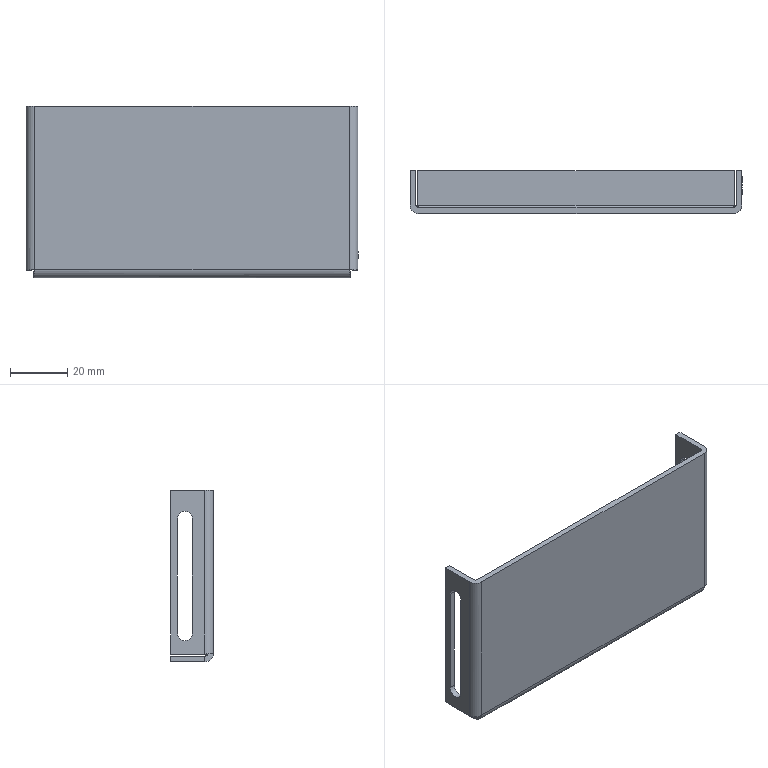Part | SolidWorks | features BaseBody 1 | 1 solid | 34 faces | box 116 x 15 x 60 mm | volume 18438 mm3 | plane 20 | cylinder 10 | spline 4 | commonest cylinder face diameters 5.2 x4 2 x3 6 x3
STEP:
#1=CARTESIAN_POINT('',(-114.,5.4,-10.));
#2=VERTEX_POINT('',#1);
#3=CARTESIAN_POINT('',(-114.,10.6,-10.));
#4=VERTEX_POINT('',#3);
#5=CARTESIAN_POINT('',(-114.,8.,-10.));
#6=DIRECTION('',(-1.,0.,0.));
#7=DIRECTION('',(0.,-1.,0.));
#8=AXIS2_PLACEMENT_3D('',#5,#6,#7);
#9=CIRCLE('',#8,2.6);
#10=EDGE_CURVE('',#2,#4,#9,.T.);
#11=ORIENTED_EDGE('',*,*,#10,.T.);
#12=CARTESIAN_POINT('',(-114.,10.6,-50.));
#13=VERTEX_POINT('',#12);
#14=CARTESIAN_POINT('',(-114.,10.6,-50.));
#15=DIRECTION('',(0.,0.,-1.));
#16=VECTOR('',#15,1000.);
#17=LINE('',#14,#16);
#18=EDGE_CURVE('',#4,#13,#17,.T.);
#19=ORIENTED_EDGE('',*,*,#18,.T.);
#20=CARTESIAN_POINT('',(-114.,5.4,-50.));
#21=VERTEX_POINT('',#20);
#22=CARTESIAN_POINT('',(-114.,8.,-50.));
#23=DIRECTION('',(-1.,0.,0.));
#24=DIRECTION('',(0.,-1.,0.));
#25=AXIS2_PLACEMENT_3D('',#22,#23,#24);
#26=CIRCLE('',#25,2.6);
#27=EDGE_CURVE('',#13,#21,#26,.T.);
#28=ORIENTED_EDGE('',*,*,#27,.T.);
#29=CARTESIAN_POINT('',(-114.,5.4,-50.));
#30=DIRECTION('',(0.,0.,1.));
#31=VECTOR('',#30,1000.);
#32=LINE('',#29,#31);
#33=EDGE_CURVE('',#21,#2,#32,.T.);
#34=ORIENTED_EDGE('',*,*,#33,.T.);
#35=EDGE_LOOP('',(#11,#19,#28,#34));
#36=FACE_BOUND('',#35,.T.);
#37=CARTESIAN_POINT('',(-114.,13.,-57.293));
#38=VERTEX_POINT('',#37);
#39=CARTESIAN_POINT('',(-114.,13.,0.));
#40=VERTEX_POINT('',#39);
#41=CARTESIAN_POINT('',(-114.,13.,-60.));
#42=DIRECTION('',(0.,0.,1.));
#43=VECTOR('',#42,1000.);
#44=LINE('',#41,#43);
#45=EDGE_CURVE('',#38,#40,#44,.T.);
#46=ORIENTED_EDGE('',*,*,#45,.T.);
#47=CARTESIAN_POINT('',(-114.,1.,0.));
#48=VERTEX_POINT('',#47);
#49=CARTESIAN_POINT('',(-114.,13.,0.));
#50=DIRECTION('',(0.,-1.,0.));
#51=VECTOR('',#50,1000.);
#52=LINE('',#49,#51);
#53=EDGE_CURVE('',#40,#48,#52,.T.);
#54=ORIENTED_EDGE('',*,*,#53,.T.);
#55=CARTESIAN_POINT('',(-114.,1.,-57.293));
#56=VERTEX_POINT('',#55);
#57=CARTESIAN_POINT('',(-114.,1.,0.));
#58=DIRECTION('',(0.,0.,-1.));
#59=VECTOR('',#58,1000.);
#60=LINE('',#57,#59);
#61=EDGE_CURVE('',#48,#56,#60,.T.);
#62=ORIENTED_EDGE('',*,*,#61,.T.);
#63=CARTESIAN_POINT('',(-114.,0.,-57.293));
#64=DIRECTION('',(0.,-1.,0.));
#65=VECTOR('',#64,1000.);
#66=LINE('',#63,#65);
#67=EDGE_CURVE('',#38,#56,#66,.T.);
#68=ORIENTED_EDGE('',*,*,#67,.F.);
#69=EDGE_LOOP('',(#46,#54,#62,#68));
#70=FACE_OUTER_BOUND('',#69,.T.);
#71=CARTESIAN_POINT('',(-114.,0.,0.));
#72=DIRECTION('',(1.,0.,0.));
#73=DIRECTION('',(0.,1.,0.));
#74=AXIS2_PLACEMENT_3D('',#71,#72,#73);
#75=PLANE('',#74);
#76=ADVANCED_FACE('',(#36,#70),#75,.T.);
#77=CARTESIAN_POINT('',(-2.,10.6,-10.));
#78=VERTEX_POINT('',#77);
#79=CARTESIAN_POINT('',(-2.,5.4,-10.));
#80=VERTEX_POINT('',#79);
#81=CARTESIAN_POINT('',(-2.,8.,-10.));
#82=DIRECTION('',(1.,0.,0.));
#83=DIRECTION('',(0.,-1.,0.));
#84=AXIS2_PLACEMENT_3D('',#81,#82,#83);
#85=CIRCLE('',#84,2.6);
#86=EDGE_CURVE('',#78,#80,#85,.T.);
#87=ORIENTED_EDGE('',*,*,#86,.T.);
#88=CARTESIAN_POINT('',(-2.,5.4,-50.));
#89=VERTEX_POINT('',#88);
#90=CARTESIAN_POINT('',(-2.,5.4,-50.));
#91=DIRECTION('',(0.,0.,-1.));
#92=VECTOR('',#91,1000.);
#93=LINE('',#90,#92);
#94=EDGE_CURVE('',#80,#89,#93,.T.);
#95=ORIENTED_EDGE('',*,*,#94,.T.);
#96=CARTESIAN_POINT('',(-2.,10.6,-50.));
#97=VERTEX_POINT('',#96);
#98=CARTESIAN_POINT('',(-2.,8.,-50.));
#99=DIRECTION('',(1.,0.,0.));
#100=DIRECTION('',(0.,-1.,0.));
#101=AXIS2_PLACEMENT_3D('',#98,#99,#100);
#102=CIRCLE('',#101,2.6);
#103=EDGE_CURVE('',#89,#97,#102,.T.);
#104=ORIENTED_EDGE('',*,*,#103,.T.);
#105=CARTESIAN_POINT('',(-2.,10.6,-50.));
#106=DIRECTION('',(0.,0.,1.));
#107=VECTOR('',#106,1000.);
#108=LINE('',#105,#107);
#109=EDGE_CURVE('',#97,#78,#108,.T.);
#110=ORIENTED_EDGE('',*,*,#109,.T.);
#111=EDGE_LOOP('',(#87,#95,#104,#110));
#112=FACE_BOUND('',#111,.T.);
#113=CARTESIAN_POINT('',(-2.,1.,0.));
#114=VERTEX_POINT('',#113);
#115=CARTESIAN_POINT('',(-2.,13.,0.));
#116=VERTEX_POINT('',#115);
#117=CARTESIAN_POINT('',(-2.,0.,0.));
#118=DIRECTION('',(0.,1.,0.));
#119=VECTOR('',#118,1000.);
#120=LINE('',#117,#119);
#121=EDGE_CURVE('',#114,#116,#120,.T.);
#122=ORIENTED_EDGE('',*,*,#121,.T.);
#123=CARTESIAN_POINT('',(-2.,13.,-57.293));
#124=VERTEX_POINT('',#123);
#125=CARTESIAN_POINT('',(-2.,13.,0.));
#126=DIRECTION('',(0.,0.,-1.));
#127=VECTOR('',#126,1000.);
#128=LINE('',#125,#127);
#129=EDGE_CURVE('',#116,#124,#128,.T.);
#130=ORIENTED_EDGE('',*,*,#129,.T.);
#131=CARTESIAN_POINT('',(-2.,1.,-57.293));
#132=VERTEX_POINT('',#131);
#133=CARTESIAN_POINT('',(-2.,0.,-57.293));
#134=DIRECTION('',(0.,-1.,0.));
#135=VECTOR('',#134,1000.);
#136=LINE('',#133,#135);
#137=EDGE_CURVE('',#124,#132,#136,.T.);
#138=ORIENTED_EDGE('',*,*,#137,.T.);
#139=CARTESIAN_POINT('',(-2.,1.,-57.293));
#140=DIRECTION('',(0.,0.,1.));
#141=VECTOR('',#140,1000.);
#142=LINE('',#139,#141);
#143=EDGE_CURVE('',#132,#114,#142,.T.);
#144=ORIENTED_EDGE('',*,*,#143,.T.);
#145=EDGE_LOOP('',(#122,#130,#138,#144));
#146=FACE_OUTER_BOUND('',#145,.T.);
#147=CARTESIAN_POINT('',(-2.,0.,0.));
#148=DIRECTION('',(-1.,0.,0.));
#149=DIRECTION('',(0.,0.,1.));
#150=AXIS2_PLACEMENT_3D('',#147,#148,#149);
#151=PLANE('',#150);
#152=ADVANCED_FACE('',(#112,#146),#151,.T.);
#153=CARTESIAN_POINT('',(-2.707,13.,-58.));
#154=VERTEX_POINT('',#153);
#155=CARTESIAN_POINT('',(-2.707,1.,-58.));
#156=VERTEX_POINT('',#155);
#157=CARTESIAN_POINT('',(-2.707,0.,-58.));
#158=DIRECTION('',(0.,-1.,0.));
#159=VECTOR('',#158,1000.);
#160=LINE('',#157,#159);
#161=EDGE_CURVE('',#154,#156,#160,.T.);
#162=ORIENTED_EDGE('',*,*,#161,.F.);
#163=CARTESIAN_POINT('',(-113.293,13.,-58.));
#164=VERTEX_POINT('',#163);
#165=CARTESIAN_POINT('',(0.,13.,-58.));
#166=DIRECTION('',(-1.,0.,0.));
#167=VECTOR('',#166,1000.);
#168=LINE('',#165,#167);
#169=EDGE_CURVE('',#154,#164,#168,.T.);
#170=ORIENTED_EDGE('',*,*,#169,.T.);
#171=CARTESIAN_POINT('',(-113.293,1.,-58.));
#172=VERTEX_POINT('',#171);
#173=CARTESIAN_POINT('',(-113.293,0.,-58.));
#174=DIRECTION('',(0.,-1.,0.));
#175=VECTOR('',#174,1000.);
#176=LINE('',#173,#175);
#177=EDGE_CURVE('',#164,#172,#176,.T.);
#178=ORIENTED_EDGE('',*,*,#177,.T.);
#179=CARTESIAN_POINT('',(-113.293,1.,-58.));
#180=DIRECTION('',(1.,0.,0.));
#181=VECTOR('',#180,1000.);
#182=LINE('',#179,#181);
#183=EDGE_CURVE('',#172,#156,#182,.T.);
#184=ORIENTED_EDGE('',*,*,#183,.T.);
#185=EDGE_LOOP('',(#162,#170,#178,#184));
#186=FACE_OUTER_BOUND('',#185,.T.);
#187=CARTESIAN_POINT('',(0.,0.,-58.));
#188=DIRECTION('',(0.,0.,1.));
#189=DIRECTION('',(0.,-1.,0.));
#190=AXIS2_PLACEMENT_3D('',#187,#188,#189);
#191=PLANE('',#190);
#192=ADVANCED_FACE('',(#186),#191,.T.);
#193=CARTESIAN_POINT('',(-116.,5.4,-10.));
#194=VERTEX_POINT('',#193);
#195=CARTESIAN_POINT('',(0.,5.4,-10.));
#196=DIRECTION('',(-1.,0.,0.));
#197=VECTOR('',#196,1000.);
#198=LINE('',#195,#197);
#199=EDGE_CURVE('',#2,#194,#198,.T.);
#200=ORIENTED_EDGE('',*,*,#199,.T.);
#201=CARTESIAN_POINT('',(-116.,10.6,-10.));
#202=VERTEX_POINT('',#201);
#203=CARTESIAN_POINT('',(-116.,8.,-10.));
#204=DIRECTION('',(-1.,0.,0.));
#205=DIRECTION('',(0.,-1.,0.));
#206=AXIS2_PLACEMENT_3D('',#203,#204,#205);
#207=CIRCLE('',#206,2.6);
#208=EDGE_CURVE('',#194,#202,#207,.T.);
#209=ORIENTED_EDGE('',*,*,#208,.T.);
#210=CARTESIAN_POINT('',(0.,10.6,-10.));
#211=DIRECTION('',(1.,0.,0.));
#212=VECTOR('',#211,1000.);
#213=LINE('',#210,#212);
#214=EDGE_CURVE('',#202,#4,#213,.T.);
#215=ORIENTED_EDGE('',*,*,#214,.T.);
#216=ORIENTED_EDGE('',*,*,#10,.F.);
#217=EDGE_LOOP('',(#200,#209,#215,#216));
#218=FACE_OUTER_BOUND('',#217,.T.);
#219=CARTESIAN_POINT('',(0.,8.,-10.));
#220=DIRECTION('',(-1.,0.,0.));
#221=DIRECTION('',(0.,-1.,0.));
#222=AXIS2_PLACEMENT_3D('',#219,#220,#221);
#223=CYLINDRICAL_SURFACE('',#222,2.6);
#224=ADVANCED_FACE('',(#218),#223,.F.);
#225=ORIENTED_EDGE('',*,*,#214,.F.);
#226=CARTESIAN_POINT('',(-116.,10.6,-50.));
#227=VERTEX_POINT('',#226);
#228=CARTESIAN_POINT('',(-116.,10.6,0.));
#229=DIRECTION('',(0.,0.,-1.));
#230=VECTOR('',#229,1000.);
#231=LINE('',#228,#230);
#232=EDGE_CURVE('',#202,#227,#231,.T.);
#233=ORIENTED_EDGE('',*,*,#232,.T.);
#234=CARTESIAN_POINT('',(0.,10.6,-50.));
#235=DIRECTION('',(1.,0.,0.));
#236=VECTOR('',#235,1000.);
#237=LINE('',#234,#236);
#238=EDGE_CURVE('',#227,#13,#237,.T.);
#239=ORIENTED_EDGE('',*,*,#238,.T.);
#240=ORIENTED_EDGE('',*,*,#18,.F.);
#241=EDGE_LOOP('',(#225,#233,#239,#240));
#242=FACE_OUTER_BOUND('',#241,.T.);
#243=CARTESIAN_POINT('',(0.,10.6,-50.));
#244=DIRECTION('',(0.,1.,0.));
#245=DIRECTION('',(1.,0.,0.));
#246=AXIS2_PLACEMENT_3D('',#243,#244,#245);
#247=PLANE('',#246);
#248=ADVANCED_FACE('',(#242),#247,.F.);
#249=ORIENTED_EDGE('',*,*,#238,.F.);
#250=CARTESIAN_POINT('',(-116.,5.4,-50.));
#251=VERTEX_POINT('',#250);
#252=CARTESIAN_POINT('',(-116.,8.,-50.));
#253=DIRECTION('',(-1.,0.,0.));
#254=DIRECTION('',(0.,-1.,0.));
#255=AXIS2_PLACEMENT_3D('',#252,#253,#254);
#256=CIRCLE('',#255,2.6);
#257=EDGE_CURVE('',#227,#251,#256,.T.);
#258=ORIENTED_EDGE('',*,*,#257,.T.);
#259=CARTESIAN_POINT('',(0.,5.4,-50.));
#260=DIRECTION('',(1.,0.,0.));
#261=VECTOR('',#260,1000.);
#262=LINE('',#259,#261);
#263=EDGE_CURVE('',#251,#21,#262,.T.);
#264=ORIENTED_EDGE('',*,*,#263,.T.);
#265=ORIENTED_EDGE('',*,*,#27,.F.);
#266=EDGE_LOOP('',(#249,#258,#264,#265));
#267=FACE_OUTER_BOUND('',#266,.T.);
#268=CARTESIAN_POINT('',(0.,8.,-50.));
#269=DIRECTION('',(-1.,0.,0.));
#270=DIRECTION('',(0.,-1.,0.));
#271=AXIS2_PLACEMENT_3D('',#268,#269,#270);
#272=CYLINDRICAL_SURFACE('',#271,2.6);
#273=ADVANCED_FACE('',(#267),#272,.F.);
#274=ORIENTED_EDGE('',*,*,#263,.F.);
#275=CARTESIAN_POINT('',(-116.,5.4,0.));
#276=DIRECTION('',(0.,0.,1.));
#277=VECTOR('',#276,1000.);
#278=LINE('',#275,#277);
#279=EDGE_CURVE('',#251,#194,#278,.T.);
#280=ORIENTED_EDGE('',*,*,#279,.T.);
#281=ORIENTED_EDGE('',*,*,#199,.F.);
#282=ORIENTED_EDGE('',*,*,#33,.F.);
#283=EDGE_LOOP('',(#274,#280,#281,#282));
#284=FACE_OUTER_BOUND('',#283,.T.);
#285=CARTESIAN_POINT('',(0.,5.4,-50.));
#286=DIRECTION('',(0.,-1.,0.));
#287=DIRECTION('',(0.,0.,-1.));
#288=AXIS2_PLACEMENT_3D('',#285,#286,#287);
#289=PLANE('',#288);
#290=ADVANCED_FACE('',(#284),#289,.F.);
#291=CARTESIAN_POINT('',(-116.,13.,-57.293));
#292=VERTEX_POINT('',#291);
#293=CARTESIAN_POINT('',(-116.,13.,0.));
#294=VERTEX_POINT('',#293);
#295=CARTESIAN_POINT('',(-116.,13.,0.));
#296=DIRECTION('',(0.,0.,1.));
#297=VECTOR('',#296,1000.);
#298=LINE('',#295,#297);
#299=EDGE_CURVE('',#292,#294,#298,.T.);
#300=ORIENTED_EDGE('',*,*,#299,.T.);
#301=CARTESIAN_POINT('',(-116.,13.,0.));
#302=DIRECTION('',(1.,0.,0.));
#303=VECTOR('',#302,1000.);
#304=LINE('',#301,#303);
#305=EDGE_CURVE('',#294,#40,#304,.T.);
#306=ORIENTED_EDGE('',*,*,#305,.T.);
#307=ORIENTED_EDGE('',*,*,#45,.F.);
#308=CARTESIAN_POINT('',(-114.,13.,-57.293));
#309=DIRECTION('',(1.,0.,0.));
#310=VECTOR('',#309,1000.);
#311=LINE('',#308,#310);
#312=EDGE_CURVE('',#292,#38,#311,.T.);
#313=ORIENTED_EDGE('',*,*,#312,.F.);
#314=EDGE_LOOP('',(#300,#306,#307,#313));
#315=FACE_OUTER_BOUND('',#314,.T.);
#316=CARTESIAN_POINT('',(-116.,13.,-60.));
#317=DIRECTION('',(0.,-1.,0.));
#318=DIRECTION('',(0.,0.,-1.));
#319=AXIS2_PLACEMENT_3D('',#316,#317,#318);
#320=PLANE('',#319);
#321=ADVANCED_FACE('',(#315),#320,.F.);
#322=ORIENTED_EDGE('',*,*,#67,.T.);
#323=CARTESIAN_POINT('',(-116.,1.,-57.293));
#324=VERTEX_POINT('',#323);
#325=CARTESIAN_POINT('',(-115.,1.,-57.293));
#326=DIRECTION('',(-1.,0.,0.));
#327=VECTOR('',#326,1000.);
#328=LINE('',#325,#327);
#329=EDGE_CURVE('',#56,#324,#328,.T.);
#330=ORIENTED_EDGE('',*,*,#329,.T.);
#331=CARTESIAN_POINT('',(-116.,0.,-57.293));
#332=DIRECTION('',(0.,1.,0.));
#333=VECTOR('',#332,1000.);
#334=LINE('',#331,#333);
#335=EDGE_CURVE('',#324,#292,#334,.T.);
#336=ORIENTED_EDGE('',*,*,#335,.T.);
#337=ORIENTED_EDGE('',*,*,#312,.T.);
#338=EDGE_LOOP('',(#322,#330,#336,#337));
#339=FACE_OUTER_BOUND('',#338,.T.);
#340=CARTESIAN_POINT('',(-114.,0.,-57.293));
#341=DIRECTION('',(0.,0.,-1.));
#342=DIRECTION('',(-1.,0.,0.));
#343=AXIS2_PLACEMENT_3D('',#340,#341,#342);
#344=PLANE('',#343);
#345=ADVANCED_FACE('',(#339),#344,.T.);
#346=CARTESIAN_POINT('',(-3.,0.,0.));
#347=VERTEX_POINT('',#346);
#348=CARTESIAN_POINT('',(-3.,1.,0.));
#349=DIRECTION('',(0.,0.,-1.));
#350=DIRECTION('',(-1.,0.,0.));
#351=AXIS2_PLACEMENT_3D('',#348,#349,#350);
#352=CIRCLE('',#351,1.);
#353=EDGE_CURVE('',#114,#347,#352,.T.);
#354=ORIENTED_EDGE('',*,*,#353,.F.);
#355=ORIENTED_EDGE('',*,*,#143,.F.);
#356=CARTESIAN_POINT('',(-3.,0.,-57.));
#357=VERTEX_POINT('',#356);
#358=CARTESIAN_POINT('',(-3.,0.,-57.));
#359=CARTESIAN_POINT('',(-2.869,0.,-57.024));
#360=CARTESIAN_POINT('',(-2.738,0.02603,-57.049));
#361=CARTESIAN_POINT('',(-2.496,0.1262,-57.098));
#362=CARTESIAN_POINT('',(-2.385,0.2003,-57.122));
#363=CARTESIAN_POINT('',(-2.2,0.3855,-57.171));
#364=CARTESIAN_POINT('',(-2.126,0.4964,-57.195));
#365=CARTESIAN_POINT('',(-2.026,0.7383,-57.244));
#366=CARTESIAN_POINT('',(-2.,0.8691,-57.268));
#367=CARTESIAN_POINT('',(-2.,1.,-57.293));
#368=B_SPLINE_CURVE_WITH_KNOTS('',3,(#358,#359,#360,#361,#362,#363,#364,#365,#366,#367),.UNSPECIFIED.,.F.,.F.,(4,2,2,2,4),(0.,0.25,0.5,0.75,1.),.UNSPECIFIED.);
#369=EDGE_CURVE('',#357,#132,#368,.T.);
#370=ORIENTED_EDGE('',*,*,#369,.F.);
#371=CARTESIAN_POINT('',(-3.,0.,0.));
#372=DIRECTION('',(0.,0.,-1.));
#373=VECTOR('',#372,1000.);
#374=LINE('',#371,#373);
#375=EDGE_CURVE('',#347,#357,#374,.T.);
#376=ORIENTED_EDGE('',*,*,#375,.F.);
#377=EDGE_LOOP('',(#354,#355,#370,#376));
#378=FACE_OUTER_BOUND('',#377,.T.);
#379=CARTESIAN_POINT('',(-3.,1.,-57.293));
#380=DIRECTION('',(0.,0.,-1.));
#381=DIRECTION('',(-1.,0.,0.));
#382=AXIS2_PLACEMENT_3D('',#379,#380,#381);
#383=CYLINDRICAL_SURFACE('',#382,1.);
#384=ADVANCED_FACE('',(#378),#383,.F.);
#385=CARTESIAN_POINT('',(-2.707,1.,-58.));
#386=CARTESIAN_POINT('',(-2.732,0.8691,-58.));
#387=CARTESIAN_POINT('',(-2.756,0.7383,-57.974));
#388=CARTESIAN_POINT('',(-2.805,0.4964,-57.874));
#389=CARTESIAN_POINT('',(-2.829,0.3855,-57.8));
#390=CARTESIAN_POINT('',(-2.878,0.2003,-57.615));
#391=CARTESIAN_POINT('',(-2.902,0.1262,-57.504));
#392=CARTESIAN_POINT('',(-2.951,0.02603,-57.262));
#393=CARTESIAN_POINT('',(-2.976,0.,-57.131));
#394=CARTESIAN_POINT('',(-3.,0.,-57.));
#395=B_SPLINE_CURVE_WITH_KNOTS('',3,(#385,#386,#387,#388,#389,#390,#391,#392,#393,#394),.UNSPECIFIED.,.F.,.F.,(4,2,2,2,4),(0.,0.25,0.5,0.75,1.),.UNSPECIFIED.);
#396=EDGE_CURVE('',#156,#357,#395,.T.);
#397=ORIENTED_EDGE('',*,*,#396,.F.);
#398=ORIENTED_EDGE('',*,*,#183,.F.);
#399=CARTESIAN_POINT('',(-113.,0.,-57.));
#400=VERTEX_POINT('',#399);
#401=CARTESIAN_POINT('',(-113.,0.,-57.));
#402=CARTESIAN_POINT('',(-113.024,0.,-57.131));
#403=CARTESIAN_POINT('',(-113.049,0.02603,-57.262));
#404=CARTESIAN_POINT('',(-113.098,0.1262,-57.504));
#405=CARTESIAN_POINT('',(-113.122,0.2003,-57.615));
#406=CARTESIAN_POINT('',(-113.171,0.3855,-57.8));
#407=CARTESIAN_POINT('',(-113.195,0.4964,-57.874));
#408=CARTESIAN_POINT('',(-113.244,0.7383,-57.974));
#409=CARTESIAN_POINT('',(-113.268,0.8691,-58.));
#410=CARTESIAN_POINT('',(-113.293,1.,-58.));
#411=B_SPLINE_CURVE_WITH_KNOTS('',3,(#401,#402,#403,#404,#405,#406,#407,#408,#409,#410),.UNSPECIFIED.,.F.,.F.,(4,2,2,2,4),(0.,0.25,0.5,0.75,1.),.UNSPECIFIED.);
#412=EDGE_CURVE('',#400,#172,#411,.T.);
#413=ORIENTED_EDGE('',*,*,#412,.F.);
#414=CARTESIAN_POINT('',(0.,0.,-57.));
#415=DIRECTION('',(-1.,0.,0.));
#416=VECTOR('',#415,1000.);
#417=LINE('',#414,#416);
#418=EDGE_CURVE('',#357,#400,#417,.T.);
#419=ORIENTED_EDGE('',*,*,#418,.F.);
#420=EDGE_LOOP('',(#397,#398,#413,#419));
#421=FACE_OUTER_BOUND('',#420,.T.);
#422=CARTESIAN_POINT('',(-113.293,1.,-57.));
#423=DIRECTION('',(-1.,0.,0.));
#424=DIRECTION('',(0.,0.,1.));
#425=AXIS2_PLACEMENT_3D('',#422,#423,#424);
#426=CYLINDRICAL_SURFACE('',#425,1.);
#427=ADVANCED_FACE('',(#421),#426,.F.);
#428=CARTESIAN_POINT('',(-113.,0.,-57.));
#429=CARTESIAN_POINT('',(-113.262,0.,-57.049));
#430=CARTESIAN_POINT('',(-113.522,0.1078,-57.098));
#431=CARTESIAN_POINT('',(-113.892,0.478,-57.195));
#432=CARTESIAN_POINT('',(-114.,0.7382,-57.244));
#433=CARTESIAN_POINT('',(-114.,1.,-57.293));
#434=B_SPLINE_CURVE_WITH_KNOTS('',3,(#428,#429,#430,#431,#432,#433),.UNSPECIFIED.,.F.,.F.,(4,2,4),(0.,0.5,1.),.UNSPECIFIED.);
#435=EDGE_CURVE('',#400,#56,#434,.T.);
#436=ORIENTED_EDGE('',*,*,#435,.T.);
#437=ORIENTED_EDGE('',*,*,#61,.F.);
#438=CARTESIAN_POINT('',(-113.,0.,0.));
#439=VERTEX_POINT('',#438);
#440=CARTESIAN_POINT('',(-113.,1.,0.));
#441=DIRECTION('',(0.,0.,-1.));
#442=DIRECTION('',(1.,0.,0.));
#443=AXIS2_PLACEMENT_3D('',#440,#441,#442);
#444=CIRCLE('',#443,1.);
#445=EDGE_CURVE('',#439,#48,#444,.T.);
#446=ORIENTED_EDGE('',*,*,#445,.F.);
#447=CARTESIAN_POINT('',(-113.,0.,0.));
#448=DIRECTION('',(0.,0.,1.));
#449=VECTOR('',#448,1000.);
#450=LINE('',#447,#449);
#451=EDGE_CURVE('',#400,#439,#450,.T.);
#452=ORIENTED_EDGE('',*,*,#451,.F.);
#453=EDGE_LOOP('',(#436,#437,#446,#452));
#454=FACE_OUTER_BOUND('',#453,.T.);
#455=CARTESIAN_POINT('',(-113.,1.,0.));
#456=DIRECTION('',(0.,0.,1.));
#457=DIRECTION('',(1.,0.,0.));
#458=AXIS2_PLACEMENT_3D('',#455,#456,#457);
#459=CYLINDRICAL_SURFACE('',#458,1.);
#460=ADVANCED_FACE('',(#454),#459,.F.);
#461=CARTESIAN_POINT('',(0.,10.6,-10.));
#462=VERTEX_POINT('',#461);
#463=CARTESIAN_POINT('',(0.,10.6,-10.));
#464=DIRECTION('',(1.,0.,0.));
#465=VECTOR('',#464,1000.);
#466=LINE('',#463,#465);
#467=EDGE_CURVE('',#78,#462,#466,.T.);
#468=ORIENTED_EDGE('',*,*,#467,.T.);
#469=CARTESIAN_POINT('',(0.,5.4,-10.));
#470=VERTEX_POINT('',#469);
#471=CARTESIAN_POINT('',(0.,8.,-10.));
#472=DIRECTION('',(1.,0.,0.));
#473=DIRECTION('',(0.,-1.,0.));
#474=AXIS2_PLACEMENT_3D('',#471,#472,#473);
#475=CIRCLE('',#474,2.6);
#476=EDGE_CURVE('',#462,#470,#475,.T.);
#477=ORIENTED_EDGE('',*,*,#476,.T.);
#478=CARTESIAN_POINT('',(0.,5.4,-10.));
#479=DIRECTION('',(-1.,0.,0.));
#480=VECTOR('',#479,1000.);
#481=LINE('',#478,#480);
#482=EDGE_CURVE('',#470,#80,#481,.T.);
#483=ORIENTED_EDGE('',*,*,#482,.T.);
#484=ORIENTED_EDGE('',*,*,#86,.F.);
#485=EDGE_LOOP('',(#468,#477,#483,#484));
#486=FACE_OUTER_BOUND('',#485,.T.);
#487=CARTESIAN_POINT('',(0.,8.,-10.));
#488=DIRECTION('',(-1.,0.,0.));
#489=DIRECTION('',(0.,-1.,0.));
#490=AXIS2_PLACEMENT_3D('',#487,#488,#489);
#491=CYLINDRICAL_SURFACE('',#490,2.6);
#492=ADVANCED_FACE('',(#486),#491,.F.);
#493=ORIENTED_EDGE('',*,*,#482,.F.);
#494=CARTESIAN_POINT('',(0.,5.4,-50.));
#495=VERTEX_POINT('',#494);
#496=CARTESIAN_POINT('',(0.,5.4,0.));
#497=DIRECTION('',(0.,0.,-1.));
#498=VECTOR('',#497,1000.);
#499=LINE('',#496,#498);
#500=EDGE_CURVE('',#470,#495,#499,.T.);
#501=ORIENTED_EDGE('',*,*,#500,.T.);
#502=CARTESIAN_POINT('',(0.,5.4,-50.));
#503=DIRECTION('',(-1.,0.,0.));
#504=VECTOR('',#503,1000.);
#505=LINE('',#502,#504);
#506=EDGE_CURVE('',#495,#89,#505,.T.);
#507=ORIENTED_EDGE('',*,*,#506,.T.);
#508=ORIENTED_EDGE('',*,*,#94,.F.);
#509=EDGE_LOOP('',(#493,#501,#507,#508));
#510=FACE_OUTER_BOUND('',#509,.T.);
#511=CARTESIAN_POINT('',(0.,5.4,-50.));
#512=DIRECTION('',(0.,-1.,0.));
#513=DIRECTION('',(0.,0.,-1.));
#514=AXIS2_PLACEMENT_3D('',#511,#512,#513);
#515=PLANE('',#514);
#516=ADVANCED_FACE('',(#510),#515,.F.);
#517=ORIENTED_EDGE('',*,*,#506,.F.);
#518=CARTESIAN_POINT('',(0.,10.6,-50.));
#519=VERTEX_POINT('',#518);
#520=CARTESIAN_POINT('',(0.,8.,-50.));
#521=DIRECTION('',(1.,0.,0.));
#522=DIRECTION('',(0.,-1.,0.));
#523=AXIS2_PLACEMENT_3D('',#520,#521,#522);
#524=CIRCLE('',#523,2.6);
#525=EDGE_CURVE('',#495,#519,#524,.T.);
#526=ORIENTED_EDGE('',*,*,#525,.T.);
#527=CARTESIAN_POINT('',(0.,10.6,-50.));
#528=DIRECTION('',(-1.,0.,0.));
#529=VECTOR('',#528,1000.);
#530=LINE('',#527,#529);
#531=EDGE_CURVE('',#519,#97,#530,.T.);
#532=ORIENTED_EDGE('',*,*,#531,.T.);
#533=ORIENTED_EDGE('',*,*,#103,.F.);
#534=EDGE_LOOP('',(#517,#526,#532,#533));
#535=FACE_OUTER_BOUND('',#534,.T.);
#536=CARTESIAN_POINT('',(0.,8.,-50.));
#537=DIRECTION('',(-1.,0.,0.));
#538=DIRECTION('',(0.,-1.,0.));
#539=AXIS2_PLACEMENT_3D('',#536,#537,#538);
#540=CYLINDRICAL_SURFACE('',#539,2.6);
#541=ADVANCED_FACE('',(#535),#540,.F.);
#542=ORIENTED_EDGE('',*,*,#531,.F.);
#543=CARTESIAN_POINT('',(0.,10.6,0.));
#544=DIRECTION('',(0.,0.,1.));
#545=VECTOR('',#544,1000.);
#546=LINE('',#543,#545);
#547=EDGE_CURVE('',#519,#462,#546,.T.);
#548=ORIENTED_EDGE('',*,*,#547,.T.);
#549=ORIENTED_EDGE('',*,*,#467,.F.);
#550=ORIENTED_EDGE('',*,*,#109,.F.);
#551=EDGE_LOOP('',(#542,#548,#549,#550));
#552=FACE_OUTER_BOUND('',#551,.T.);
#553=CARTESIAN_POINT('',(0.,10.6,-50.));
#554=DIRECTION('',(0.,1.,0.));
#555=DIRECTION('',(1.,0.,0.));
#556=AXIS2_PLACEMENT_3D('',#553,#554,#555);
#557=PLANE('',#556);
#558=ADVANCED_FACE('',(#552),#557,.F.);
#559=CARTESIAN_POINT('',(0.,13.,-57.293));
#560=VERTEX_POINT('',#559);
#561=CARTESIAN_POINT('',(-2.,13.,-57.293));
#562=DIRECTION('',(-1.,0.,0.));
#563=VECTOR('',#562,1000.);
#564=LINE('',#561,#563);
#565=EDGE_CURVE('',#560,#124,#564,.T.);
#566=ORIENTED_EDGE('',*,*,#565,.T.);
#567=ORIENTED_EDGE('',*,*,#129,.F.);
#568=CARTESIAN_POINT('',(0.,13.,0.));
#569=VERTEX_POINT('',#568);
#570=CARTESIAN_POINT('',(0.,13.,0.));
#571=DIRECTION('',(1.,0.,0.));
#572=VECTOR('',#571,1000.);
#573=LINE('',#570,#572);
#574=EDGE_CURVE('',#116,#569,#573,.T.);
#575=ORIENTED_EDGE('',*,*,#574,.T.);
#576=CARTESIAN_POINT('',(0.,13.,0.));
#577=DIRECTION('',(0.,0.,-1.));
#578=VECTOR('',#577,1000.);
#579=LINE('',#576,#578);
#580=EDGE_CURVE('',#569,#560,#579,.T.);
#581=ORIENTED_EDGE('',*,*,#580,.T.);
#582=EDGE_LOOP('',(#566,#567,#575,#581));
#583=FACE_OUTER_BOUND('',#582,.T.);
#584=CARTESIAN_POINT('',(0.,13.,0.));
#585=DIRECTION('',(0.,-1.,0.));
#586=DIRECTION('',(-1.,0.,0.));
#587=AXIS2_PLACEMENT_3D('',#584,#585,#586);
#588=PLANE('',#587);
#589=ADVANCED_FACE('',(#583),#588,.F.);
#590=CARTESIAN_POINT('',(0.,1.,-57.293));
#591=VERTEX_POINT('',#590);
#592=CARTESIAN_POINT('',(0.,0.,-57.293));
#593=DIRECTION('',(0.,-1.,0.));
#594=VECTOR('',#593,1000.);
#595=LINE('',#592,#594);
#596=EDGE_CURVE('',#560,#591,#595,.T.);
#597=ORIENTED_EDGE('',*,*,#596,.T.);
#598=CARTESIAN_POINT('',(-1.,1.,-57.293));
#599=DIRECTION('',(-1.,0.,0.));
#600=VECTOR('',#599,1000.);
#601=LINE('',#598,#600);
#602=EDGE_CURVE('',#591,#132,#601,.T.);
#603=ORIENTED_EDGE('',*,*,#602,.T.);
#604=ORIENTED_EDGE('',*,*,#137,.F.);
#605=ORIENTED_EDGE('',*,*,#565,.F.);
#606=EDGE_LOOP('',(#597,#603,#604,#605));
#607=FACE_OUTER_BOUND('',#606,.T.);
#608=CARTESIAN_POINT('',(-2.,0.,-57.293));
#609=DIRECTION('',(0.,0.,1.));
#610=DIRECTION('',(0.,-1.,0.));
#611=AXIS2_PLACEMENT_3D('',#608,#609,#610);
#612=PLANE('',#611);
#613=ADVANCED_FACE('',(#607),#612,.F.);
#614=CARTESIAN_POINT('',(-113.293,13.,-60.));
#615=VERTEX_POINT('',#614);
#616=CARTESIAN_POINT('',(-113.293,13.,-58.));
#617=DIRECTION('',(0.,0.,1.));
#618=VECTOR('',#617,1000.);
#619=LINE('',#616,#618);
#620=EDGE_CURVE('',#615,#164,#619,.T.);
#621=ORIENTED_EDGE('',*,*,#620,.T.);
#622=ORIENTED_EDGE('',*,*,#169,.F.);
#623=CARTESIAN_POINT('',(-2.707,13.,-60.));
#624=VERTEX_POINT('',#623);
#625=CARTESIAN_POINT('',(-2.707,13.,-58.));
#626=DIRECTION('',(0.,0.,1.));
#627=VECTOR('',#626,1000.);
#628=LINE('',#625,#627);
#629=EDGE_CURVE('',#624,#154,#628,.T.);
#630=ORIENTED_EDGE('',*,*,#629,.F.);
#631=CARTESIAN_POINT('',(0.,13.,-60.));
#632=DIRECTION('',(-1.,0.,0.));
#633=VECTOR('',#632,1000.);
#634=LINE('',#631,#633);
#635=EDGE_CURVE('',#624,#615,#634,.T.);
#636=ORIENTED_EDGE('',*,*,#635,.T.);
#637=EDGE_LOOP('',(#621,#622,#630,#636));
#638=FACE_OUTER_BOUND('',#637,.T.);
#639=CARTESIAN_POINT('',(0.,13.,-60.));
#640=DIRECTION('',(0.,-1.,0.));
#641=DIRECTION('',(-1.,0.,0.));
#642=AXIS2_PLACEMENT_3D('',#639,#640,#641);
#643=PLANE('',#642);
#644=ADVANCED_FACE('',(#638),#643,.F.);
#645=CARTESIAN_POINT('',(-113.293,1.,-60.));
#646=VERTEX_POINT('',#645);
#647=CARTESIAN_POINT('',(-113.293,0.,-60.));
#648=DIRECTION('',(0.,-1.,0.));
#649=VECTOR('',#648,1000.);
#650=LINE('',#647,#649);
#651=EDGE_CURVE('',#615,#646,#650,.T.);
#652=ORIENTED_EDGE('',*,*,#651,.T.);
#653=CARTESIAN_POINT('',(-113.293,1.,-59.));
#654=DIRECTION('',(0.,0.,1.));
#655=VECTOR('',#654,1000.);
#656=LINE('',#653,#655);
#657=EDGE_CURVE('',#646,#172,#656,.T.);
#658=ORIENTED_EDGE('',*,*,#657,.T.);
#659=ORIENTED_EDGE('',*,*,#177,.F.);
#660=ORIENTED_EDGE('',*,*,#620,.F.);
#661=EDGE_LOOP('',(#652,#658,#659,#660));
#662=FACE_OUTER_BOUND('',#661,.T.);
#663=CARTESIAN_POINT('',(-113.293,0.,-58.));
#664=DIRECTION('',(1.,0.,0.));
#665=DIRECTION('',(0.,-1.,0.));
#666=AXIS2_PLACEMENT_3D('',#663,#664,#665);
#667=PLANE('',#666);
#668=ADVANCED_FACE('',(#662),#667,.F.);
#669=ORIENTED_EDGE('',*,*,#161,.T.);
#670=CARTESIAN_POINT('',(-2.707,1.,-60.));
#671=VERTEX_POINT('',#670);
#672=CARTESIAN_POINT('',(-2.707,1.,-59.));
#673=DIRECTION('',(0.,0.,-1.));
#674=VECTOR('',#673,1000.);
#675=LINE('',#672,#674);
#676=EDGE_CURVE('',#156,#671,#675,.T.);
#677=ORIENTED_EDGE('',*,*,#676,.T.);
#678=CARTESIAN_POINT('',(-2.707,0.,-60.));
#679=DIRECTION('',(0.,1.,0.));
#680=VECTOR('',#679,1000.);
#681=LINE('',#678,#680);
#682=EDGE_CURVE('',#671,#624,#681,.T.);
#683=ORIENTED_EDGE('',*,*,#682,.T.);
#684=ORIENTED_EDGE('',*,*,#629,.T.);
#685=EDGE_LOOP('',(#669,#677,#683,#684));
#686=FACE_OUTER_BOUND('',#685,.T.);
#687=CARTESIAN_POINT('',(-2.707,0.,-58.));
#688=DIRECTION('',(1.,0.,0.));
#689=DIRECTION('',(0.,0.,-1.));
#690=AXIS2_PLACEMENT_3D('',#687,#688,#689);
#691=PLANE('',#690);
#692=ADVANCED_FACE('',(#686),#691,.T.);
#693=ORIENTED_EDGE('',*,*,#257,.F.);
#694=ORIENTED_EDGE('',*,*,#232,.F.);
#695=ORIENTED_EDGE('',*,*,#208,.F.);
#696=ORIENTED_EDGE('',*,*,#279,.F.);
#697=EDGE_LOOP('',(#693,#694,#695,#696));
#698=FACE_BOUND('',#697,.T.);
#699=CARTESIAN_POINT('',(-116.,1.,0.));
#700=VERTEX_POINT('',#699);
#701=CARTESIAN_POINT('',(-116.,1.,0.));
#702=DIRECTION('',(0.,0.,-1.));
#703=VECTOR('',#702,1000.);
#704=LINE('',#701,#703);
#705=EDGE_CURVE('',#700,#324,#704,.T.);
#706=ORIENTED_EDGE('',*,*,#705,.F.);
#707=CARTESIAN_POINT('',(-116.,0.,0.));
#708=DIRECTION('',(0.,-1.,0.));
#709=VECTOR('',#708,1000.);
#710=LINE('',#707,#709);
#711=EDGE_CURVE('',#294,#700,#710,.T.);
#712=ORIENTED_EDGE('',*,*,#711,.F.);
#713=ORIENTED_EDGE('',*,*,#299,.F.);
#714=ORIENTED_EDGE('',*,*,#335,.F.);
#715=EDGE_LOOP('',(#706,#712,#713,#714));
#716=FACE_OUTER_BOUND('',#715,.T.);
#717=CARTESIAN_POINT('',(-116.,0.,0.));
#718=DIRECTION('',(1.,0.,0.));
#719=DIRECTION('',(0.,1.,0.));
#720=AXIS2_PLACEMENT_3D('',#717,#718,#719);
#721=PLANE('',#720);
#722=ADVANCED_FACE('',(#698,#716),#721,.F.);
#723=ORIENTED_EDGE('',*,*,#435,.F.);
#724=CARTESIAN_POINT('',(-113.,-2.,-57.));
#725=VERTEX_POINT('',#724);
#726=CARTESIAN_POINT('',(-113.,-0.9999,-57.));
#727=DIRECTION('',(0.,-1.,0.));
#728=VECTOR('',#727,1000.);
#729=LINE('',#726,#728);
#730=EDGE_CURVE('',#400,#725,#729,.T.);
#731=ORIENTED_EDGE('',*,*,#730,.T.);
#732=CARTESIAN_POINT('',(-116.,1.,-57.293));
#733=CARTESIAN_POINT('',(-116.,0.6073,-57.268));
#734=CARTESIAN_POINT('',(-115.922,0.2148,-57.244));
#735=CARTESIAN_POINT('',(-115.621,-0.5109,-57.195));
#736=CARTESIAN_POINT('',(-115.399,-0.8436,-57.171));
#737=CARTESIAN_POINT('',(-114.844,-1.399,-57.122));
#738=CARTESIAN_POINT('',(-114.511,-1.621,-57.098));
#739=CARTESIAN_POINT('',(-113.785,-1.922,-57.049));
#740=CARTESIAN_POINT('',(-113.393,-2.,-57.024));
#741=CARTESIAN_POINT('',(-113.,-2.,-57.));
#742=B_SPLINE_CURVE_WITH_KNOTS('',3,(#732,#733,#734,#735,#736,#737,#738,#739,#740,#741),.UNSPECIFIED.,.F.,.F.,(4,2,2,2,4),(0.,0.25,0.5,0.75,1.),.UNSPECIFIED.);
#743=EDGE_CURVE('',#324,#725,#742,.T.);
#744=ORIENTED_EDGE('',*,*,#743,.F.);
#745=ORIENTED_EDGE('',*,*,#329,.F.);
#746=EDGE_LOOP('',(#723,#731,#744,#745));
#747=FACE_OUTER_BOUND('',#746,.T.);
#748=CARTESIAN_POINT('',(-113.,-2.02,-57.));
#749=CARTESIAN_POINT('',(-113.395,-2.02,-57.024));
#750=CARTESIAN_POINT('',(-113.79,-1.941,-57.049));
#751=CARTESIAN_POINT('',(-114.521,-1.639,-57.098));
#752=CARTESIAN_POINT('',(-114.856,-1.415,-57.122));
#753=CARTESIAN_POINT('',(-115.415,-0.8559,-57.171));
#754=CARTESIAN_POINT('',(-115.639,-0.5209,-57.195));
#755=CARTESIAN_POINT('',(-115.941,0.2095,-57.244));
#756=CARTESIAN_POINT('',(-116.02,0.6046,-57.268));
#757=CARTESIAN_POINT('',(-116.02,1.,-57.293));
#758=CARTESIAN_POINT('',(-113.,-2.,-57.));
#759=CARTESIAN_POINT('',(-113.393,-2.,-57.024));
#760=CARTESIAN_POINT('',(-113.785,-1.922,-57.049));
#761=CARTESIAN_POINT('',(-114.511,-1.621,-57.098));
#762=CARTESIAN_POINT('',(-114.844,-1.399,-57.122));
#763=CARTESIAN_POINT('',(-115.399,-0.8436,-57.171));
#764=CARTESIAN_POINT('',(-115.621,-0.5109,-57.195));
#765=CARTESIAN_POINT('',(-115.922,0.2148,-57.244));
#766=CARTESIAN_POINT('',(-116.,0.6072,-57.268));
#767=CARTESIAN_POINT('',(-116.,1.,-57.293));
#768=CARTESIAN_POINT('',(-113.,0.,-57.));
#769=CARTESIAN_POINT('',(-113.131,0.,-57.024));
#770=CARTESIAN_POINT('',(-113.262,0.02603,-57.049));
#771=CARTESIAN_POINT('',(-113.504,0.1262,-57.098));
#772=CARTESIAN_POINT('',(-113.615,0.2003,-57.122));
#773=CARTESIAN_POINT('',(-113.8,0.3855,-57.171));
#774=CARTESIAN_POINT('',(-113.874,0.4964,-57.195));
#775=CARTESIAN_POINT('',(-113.974,0.7383,-57.244));
#776=CARTESIAN_POINT('',(-114.,0.8691,-57.268));
#777=CARTESIAN_POINT('',(-114.,1.,-57.293));
#778=CARTESIAN_POINT('',(-113.,0.0202,-57.));
#779=CARTESIAN_POINT('',(-113.128,0.0202,-57.024));
#780=CARTESIAN_POINT('',(-113.256,0.0457,-57.049));
#781=CARTESIAN_POINT('',(-113.493,0.1439,-57.098));
#782=CARTESIAN_POINT('',(-113.602,0.2165,-57.122));
#783=CARTESIAN_POINT('',(-113.784,0.3979,-57.171));
#784=CARTESIAN_POINT('',(-113.856,0.5066,-57.195));
#785=CARTESIAN_POINT('',(-113.954,0.7435,-57.244));
#786=CARTESIAN_POINT('',(-113.98,0.8717,-57.268));
#787=CARTESIAN_POINT('',(-113.98,1.,-57.293));
#788=B_SPLINE_SURFACE_WITH_KNOTS('',1,3,((#748,#749,#750,#751,#752,#753,#754,#755,#756,#757),(#758,#759,#760,#761,#762,#763,#764,#765,#766,#767),(#768,#769,#770,#771,#772,#773,#774,#775,#776,#777),(#778,#779,#780,#781,#782,#783,#784,#785,#786,#787)),.UNSPECIFIED.,.F.,.F.,.F.,(2,1,1,2),(4,2,2,2,4),(-0.01,0.,1.,1.01),(0.,0.25,0.5,0.75,1.),.UNSPECIFIED.);
#789=ADVANCED_FACE('',(#747),#788,.F.);
#790=ORIENTED_EDGE('',*,*,#451,.T.);
#791=CARTESIAN_POINT('',(0.,0.,0.));
#792=DIRECTION('',(-1.,0.,0.));
#793=VECTOR('',#792,1000.);
#794=LINE('',#791,#793);
#795=EDGE_CURVE('',#347,#439,#794,.T.);
#796=ORIENTED_EDGE('',*,*,#795,.F.);
#797=ORIENTED_EDGE('',*,*,#375,.T.);
#798=ORIENTED_EDGE('',*,*,#418,.T.);
#799=EDGE_LOOP('',(#790,#796,#797,#798));
#800=FACE_OUTER_BOUND('',#799,.T.);
#801=CARTESIAN_POINT('',(0.,0.,0.));
#802=DIRECTION('',(0.,1.,0.));
#803=DIRECTION('',(1.,0.,0.));
#804=AXIS2_PLACEMENT_3D('',#801,#802,#803);
#805=PLANE('',#804);
#806=ADVANCED_FACE('',(#800),#805,.T.);
#807=ORIENTED_EDGE('',*,*,#602,.F.);
#808=CARTESIAN_POINT('',(-3.,-2.,-57.));
#809=VERTEX_POINT('',#808);
#810=CARTESIAN_POINT('',(-3.,-2.,-57.));
#811=CARTESIAN_POINT('',(-2.607,-2.,-57.024));
#812=CARTESIAN_POINT('',(-2.215,-1.922,-57.049));
#813=CARTESIAN_POINT('',(-1.489,-1.621,-57.098));
#814=CARTESIAN_POINT('',(-1.156,-1.399,-57.122));
#815=CARTESIAN_POINT('',(-0.601,-0.8436,-57.171));
#816=CARTESIAN_POINT('',(-0.3786,-0.5109,-57.195));
#817=CARTESIAN_POINT('',(-0.07808,0.2148,-57.244));
#818=CARTESIAN_POINT('',(0.,0.6073,-57.268));
#819=CARTESIAN_POINT('',(0.,1.,-57.293));
#820=B_SPLINE_CURVE_WITH_KNOTS('',3,(#810,#811,#812,#813,#814,#815,#816,#817,#818,#819),.UNSPECIFIED.,.F.,.F.,(4,2,2,2,4),(0.,0.25,0.5,0.75,1.),.UNSPECIFIED.);
#821=EDGE_CURVE('',#809,#591,#820,.T.);
#822=ORIENTED_EDGE('',*,*,#821,.F.);
#823=CARTESIAN_POINT('',(-3.,-0.9999,-57.));
#824=DIRECTION('',(0.,1.,0.));
#825=VECTOR('',#824,1000.);
#826=LINE('',#823,#825);
#827=EDGE_CURVE('',#809,#357,#826,.T.);
#828=ORIENTED_EDGE('',*,*,#827,.T.);
#829=ORIENTED_EDGE('',*,*,#369,.T.);
#830=EDGE_LOOP('',(#807,#822,#828,#829));
#831=FACE_OUTER_BOUND('',#830,.T.);
#832=CARTESIAN_POINT('',(0.02,1.,-57.293));
#833=CARTESIAN_POINT('',(0.02,0.6046,-57.268));
#834=CARTESIAN_POINT('',(-0.0586,0.2095,-57.244));
#835=CARTESIAN_POINT('',(-0.3612,-0.5209,-57.195));
#836=CARTESIAN_POINT('',(-0.585,-0.8559,-57.171));
#837=CARTESIAN_POINT('',(-1.144,-1.415,-57.122));
#838=CARTESIAN_POINT('',(-1.479,-1.639,-57.098));
#839=CARTESIAN_POINT('',(-2.21,-1.941,-57.049));
#840=CARTESIAN_POINT('',(-2.605,-2.02,-57.024));
#841=CARTESIAN_POINT('',(-3.,-2.02,-57.));
#842=CARTESIAN_POINT('',(0.,1.,-57.293));
#843=CARTESIAN_POINT('',(0.,0.6072,-57.268));
#844=CARTESIAN_POINT('',(-0.07808,0.2148,-57.244));
#845=CARTESIAN_POINT('',(-0.3786,-0.5109,-57.195));
#846=CARTESIAN_POINT('',(-0.601,-0.8436,-57.171));
#847=CARTESIAN_POINT('',(-1.156,-1.399,-57.122));
#848=CARTESIAN_POINT('',(-1.489,-1.621,-57.098));
#849=CARTESIAN_POINT('',(-2.215,-1.922,-57.049));
#850=CARTESIAN_POINT('',(-2.607,-2.,-57.024));
#851=CARTESIAN_POINT('',(-3.,-2.,-57.));
#852=CARTESIAN_POINT('',(-2.,1.,-57.293));
#853=CARTESIAN_POINT('',(-2.,0.8691,-57.268));
#854=CARTESIAN_POINT('',(-2.026,0.7383,-57.244));
#855=CARTESIAN_POINT('',(-2.126,0.4964,-57.195));
#856=CARTESIAN_POINT('',(-2.2,0.3855,-57.171));
#857=CARTESIAN_POINT('',(-2.385,0.2003,-57.122));
#858=CARTESIAN_POINT('',(-2.496,0.1262,-57.098));
#859=CARTESIAN_POINT('',(-2.738,0.02603,-57.049));
#860=CARTESIAN_POINT('',(-2.869,0.,-57.024));
#861=CARTESIAN_POINT('',(-3.,0.,-57.));
#862=CARTESIAN_POINT('',(-2.02,1.,-57.293));
#863=CARTESIAN_POINT('',(-2.02,0.8717,-57.268));
#864=CARTESIAN_POINT('',(-2.046,0.7435,-57.244));
#865=CARTESIAN_POINT('',(-2.144,0.5066,-57.195));
#866=CARTESIAN_POINT('',(-2.216,0.3979,-57.171));
#867=CARTESIAN_POINT('',(-2.398,0.2165,-57.122));
#868=CARTESIAN_POINT('',(-2.507,0.1439,-57.098));
#869=CARTESIAN_POINT('',(-2.744,0.0457,-57.049));
#870=CARTESIAN_POINT('',(-2.872,0.0202,-57.024));
#871=CARTESIAN_POINT('',(-3.,0.0202,-57.));
#872=B_SPLINE_SURFACE_WITH_KNOTS('',1,3,((#832,#833,#834,#835,#836,#837,#838,#839,#840,#841),(#842,#843,#844,#845,#846,#847,#848,#849,#850,#851),(#852,#853,#854,#855,#856,#857,#858,#859,#860,#861),(#862,#863,#864,#865,#866,#867,#868,#869,#870,#871)),.UNSPECIFIED.,.F.,.F.,.F.,(2,1,1,2),(4,2,2,2,4),(-0.01,0.,1.,1.01),(0.,0.25,0.5,0.75,1.),.UNSPECIFIED.);
#873=ADVANCED_FACE('',(#831),#872,.F.);
#874=ORIENTED_EDGE('',*,*,#525,.F.);
#875=ORIENTED_EDGE('',*,*,#500,.F.);
#876=ORIENTED_EDGE('',*,*,#476,.F.);
#877=ORIENTED_EDGE('',*,*,#547,.F.);
#878=EDGE_LOOP('',(#874,#875,#876,#877));
#879=FACE_BOUND('',#878,.T.);
#880=ORIENTED_EDGE('',*,*,#596,.F.);
#881=ORIENTED_EDGE('',*,*,#580,.F.);
#882=CARTESIAN_POINT('',(0.,1.,0.));
#883=VERTEX_POINT('',#882);
#884=CARTESIAN_POINT('',(0.,0.,0.));
#885=DIRECTION('',(0.,1.,0.));
#886=VECTOR('',#885,1000.);
#887=LINE('',#884,#886);
#888=EDGE_CURVE('',#883,#569,#887,.T.);
#889=ORIENTED_EDGE('',*,*,#888,.F.);
#890=CARTESIAN_POINT('',(0.,1.,-57.293));
#891=DIRECTION('',(0.,0.,1.));
#892=VECTOR('',#891,1000.);
#893=LINE('',#890,#892);
#894=EDGE_CURVE('',#591,#883,#893,.T.);
#895=ORIENTED_EDGE('',*,*,#894,.F.);
#896=EDGE_LOOP('',(#880,#881,#889,#895));
#897=FACE_OUTER_BOUND('',#896,.T.);
#898=CARTESIAN_POINT('',(0.,0.,0.));
#899=DIRECTION('',(-1.,0.,0.));
#900=DIRECTION('',(0.,0.,1.));
#901=AXIS2_PLACEMENT_3D('',#898,#899,#900);
#902=PLANE('',#901);
#903=ADVANCED_FACE('',(#879,#897),#902,.F.);
#904=ORIENTED_EDGE('',*,*,#657,.F.);
#905=CARTESIAN_POINT('',(-113.,-2.,-57.));
#906=CARTESIAN_POINT('',(-113.024,-2.,-57.393));
#907=CARTESIAN_POINT('',(-113.049,-1.922,-57.785));
#908=CARTESIAN_POINT('',(-113.098,-1.621,-58.511));
#909=CARTESIAN_POINT('',(-113.122,-1.399,-58.844));
#910=CARTESIAN_POINT('',(-113.171,-0.8436,-59.399));
#911=CARTESIAN_POINT('',(-113.195,-0.5109,-59.621));
#912=CARTESIAN_POINT('',(-113.244,0.2148,-59.922));
#913=CARTESIAN_POINT('',(-113.268,0.6073,-60.));
#914=CARTESIAN_POINT('',(-113.293,1.,-60.));
#915=B_SPLINE_CURVE_WITH_KNOTS('',3,(#905,#906,#907,#908,#909,#910,#911,#912,#913,#914),.UNSPECIFIED.,.F.,.F.,(4,2,2,2,4),(0.,0.25,0.5,0.75,1.),.UNSPECIFIED.);
#916=EDGE_CURVE('',#725,#646,#915,.T.);
#917=ORIENTED_EDGE('',*,*,#916,.F.);
#918=ORIENTED_EDGE('',*,*,#730,.F.);
#919=ORIENTED_EDGE('',*,*,#412,.T.);
#920=EDGE_LOOP('',(#904,#917,#918,#919));
#921=FACE_OUTER_BOUND('',#920,.T.);
#922=CARTESIAN_POINT('',(-113.293,1.,-60.02));
#923=CARTESIAN_POINT('',(-113.268,0.6046,-60.02));
#924=CARTESIAN_POINT('',(-113.244,0.2095,-59.941));
#925=CARTESIAN_POINT('',(-113.195,-0.5209,-59.639));
#926=CARTESIAN_POINT('',(-113.171,-0.8559,-59.415));
#927=CARTESIAN_POINT('',(-113.122,-1.415,-58.856));
#928=CARTESIAN_POINT('',(-113.098,-1.639,-58.521));
#929=CARTESIAN_POINT('',(-113.049,-1.941,-57.79));
#930=CARTESIAN_POINT('',(-113.024,-2.02,-57.395));
#931=CARTESIAN_POINT('',(-113.,-2.02,-57.));
#932=CARTESIAN_POINT('',(-113.293,1.,-60.));
#933=CARTESIAN_POINT('',(-113.268,0.6072,-60.));
#934=CARTESIAN_POINT('',(-113.244,0.2148,-59.922));
#935=CARTESIAN_POINT('',(-113.195,-0.5109,-59.621));
#936=CARTESIAN_POINT('',(-113.171,-0.8436,-59.399));
#937=CARTESIAN_POINT('',(-113.122,-1.399,-58.844));
#938=CARTESIAN_POINT('',(-113.098,-1.621,-58.511));
#939=CARTESIAN_POINT('',(-113.049,-1.922,-57.785));
#940=CARTESIAN_POINT('',(-113.024,-2.,-57.393));
#941=CARTESIAN_POINT('',(-113.,-2.,-57.));
#942=CARTESIAN_POINT('',(-113.293,1.,-58.));
#943=CARTESIAN_POINT('',(-113.268,0.8691,-58.));
#944=CARTESIAN_POINT('',(-113.244,0.7383,-57.974));
#945=CARTESIAN_POINT('',(-113.195,0.4964,-57.874));
#946=CARTESIAN_POINT('',(-113.171,0.3855,-57.8));
#947=CARTESIAN_POINT('',(-113.122,0.2003,-57.615));
#948=CARTESIAN_POINT('',(-113.098,0.1262,-57.504));
#949=CARTESIAN_POINT('',(-113.049,0.02603,-57.262));
#950=CARTESIAN_POINT('',(-113.024,0.,-57.131));
#951=CARTESIAN_POINT('',(-113.,0.,-57.));
#952=CARTESIAN_POINT('',(-113.293,1.,-57.98));
#953=CARTESIAN_POINT('',(-113.268,0.8717,-57.98));
#954=CARTESIAN_POINT('',(-113.244,0.7435,-57.954));
#955=CARTESIAN_POINT('',(-113.195,0.5066,-57.856));
#956=CARTESIAN_POINT('',(-113.171,0.3979,-57.784));
#957=CARTESIAN_POINT('',(-113.122,0.2165,-57.602));
#958=CARTESIAN_POINT('',(-113.098,0.1439,-57.493));
#959=CARTESIAN_POINT('',(-113.049,0.0457,-57.256));
#960=CARTESIAN_POINT('',(-113.024,0.0202,-57.128));
#961=CARTESIAN_POINT('',(-113.,0.0202,-57.));
#962=B_SPLINE_SURFACE_WITH_KNOTS('',1,3,((#922,#923,#924,#925,#926,#927,#928,#929,#930,#931),(#932,#933,#934,#935,#936,#937,#938,#939,#940,#941),(#942,#943,#944,#945,#946,#947,#948,#949,#950,#951),(#952,#953,#954,#955,#956,#957,#958,#959,#960,#961)),.UNSPECIFIED.,.F.,.F.,.F.,(2,1,1,2),(4,2,2,2,4),(-0.01,0.,1.,1.01),(0.,0.25,0.5,0.75,1.),.UNSPECIFIED.);
#963=ADVANCED_FACE('',(#921),#962,.F.);
#964=ORIENTED_EDGE('',*,*,#651,.F.);
#965=ORIENTED_EDGE('',*,*,#635,.F.);
#966=ORIENTED_EDGE('',*,*,#682,.F.);
#967=CARTESIAN_POINT('',(-113.293,1.,-60.));
#968=DIRECTION('',(1.,0.,0.));
#969=VECTOR('',#968,1000.);
#970=LINE('',#967,#969);
#971=EDGE_CURVE('',#646,#671,#970,.T.);
#972=ORIENTED_EDGE('',*,*,#971,.F.);
#973=EDGE_LOOP('',(#964,#965,#966,#972));
#974=FACE_OUTER_BOUND('',#973,.T.);
#975=CARTESIAN_POINT('',(0.,0.,-60.));
#976=DIRECTION('',(0.,0.,1.));
#977=DIRECTION('',(0.,-1.,0.));
#978=AXIS2_PLACEMENT_3D('',#975,#976,#977);
#979=PLANE('',#978);
#980=ADVANCED_FACE('',(#974),#979,.F.);
#981=ORIENTED_EDGE('',*,*,#396,.T.);
#982=ORIENTED_EDGE('',*,*,#827,.F.);
#983=CARTESIAN_POINT('',(-2.707,1.,-60.));
#984=CARTESIAN_POINT('',(-2.732,0.6073,-60.));
#985=CARTESIAN_POINT('',(-2.756,0.2148,-59.922));
#986=CARTESIAN_POINT('',(-2.805,-0.5109,-59.621));
#987=CARTESIAN_POINT('',(-2.829,-0.8436,-59.399));
#988=CARTESIAN_POINT('',(-2.878,-1.399,-58.844));
#989=CARTESIAN_POINT('',(-2.902,-1.621,-58.511));
#990=CARTESIAN_POINT('',(-2.951,-1.922,-57.785));
#991=CARTESIAN_POINT('',(-2.976,-2.,-57.393));
#992=CARTESIAN_POINT('',(-3.,-2.,-57.));
#993=B_SPLINE_CURVE_WITH_KNOTS('',3,(#983,#984,#985,#986,#987,#988,#989,#990,#991,#992),.UNSPECIFIED.,.F.,.F.,(4,2,2,2,4),(0.,0.25,0.5,0.75,1.),.UNSPECIFIED.);
#994=EDGE_CURVE('',#671,#809,#993,.T.);
#995=ORIENTED_EDGE('',*,*,#994,.F.);
#996=ORIENTED_EDGE('',*,*,#676,.F.);
#997=EDGE_LOOP('',(#981,#982,#995,#996));
#998=FACE_OUTER_BOUND('',#997,.T.);
#999=CARTESIAN_POINT('',(-3.,-2.02,-57.));
#1000=CARTESIAN_POINT('',(-2.976,-2.02,-57.395));
#1001=CARTESIAN_POINT('',(-2.951,-1.941,-57.79));
#1002=CARTESIAN_POINT('',(-2.902,-1.639,-58.521));
#1003=CARTESIAN_POINT('',(-2.878,-1.415,-58.856));
#1004=CARTESIAN_POINT('',(-2.829,-0.8559,-59.415));
#1005=CARTESIAN_POINT('',(-2.805,-0.5209,-59.639));
#1006=CARTESIAN_POINT('',(-2.756,0.2095,-59.941));
#1007=CARTESIAN_POINT('',(-2.732,0.6046,-60.02));
#1008=CARTESIAN_POINT('',(-2.707,1.,-60.02));
#1009=CARTESIAN_POINT('',(-3.,-2.,-57.));
#1010=CARTESIAN_POINT('',(-2.976,-2.,-57.393));
#1011=CARTESIAN_POINT('',(-2.951,-1.922,-57.785));
#1012=CARTESIAN_POINT('',(-2.902,-1.621,-58.511));
#1013=CARTESIAN_POINT('',(-2.878,-1.399,-58.844));
#1014=CARTESIAN_POINT('',(-2.829,-0.8436,-59.399));
#1015=CARTESIAN_POINT('',(-2.805,-0.5109,-59.621));
#1016=CARTESIAN_POINT('',(-2.756,0.2148,-59.922));
#1017=CARTESIAN_POINT('',(-2.732,0.6072,-60.));
#1018=CARTESIAN_POINT('',(-2.707,1.,-60.));
#1019=CARTESIAN_POINT('',(-3.,0.,-57.));
#1020=CARTESIAN_POINT('',(-2.976,0.,-57.131));
#1021=CARTESIAN_POINT('',(-2.951,0.02603,-57.262));
#1022=CARTESIAN_POINT('',(-2.902,0.1262,-57.504));
#1023=CARTESIAN_POINT('',(-2.878,0.2003,-57.615));
#1024=CARTESIAN_POINT('',(-2.829,0.3855,-57.8));
#1025=CARTESIAN_POINT('',(-2.805,0.4964,-57.874));
#1026=CARTESIAN_POINT('',(-2.756,0.7383,-57.974));
#1027=CARTESIAN_POINT('',(-2.732,0.8691,-58.));
#1028=CARTESIAN_POINT('',(-2.707,1.,-58.));
#1029=CARTESIAN_POINT('',(-3.,0.0202,-57.));
#1030=CARTESIAN_POINT('',(-2.976,0.0202,-57.128));
#1031=CARTESIAN_POINT('',(-2.951,0.0457,-57.256));
#1032=CARTESIAN_POINT('',(-2.902,0.1439,-57.493));
#1033=CARTESIAN_POINT('',(-2.878,0.2165,-57.602));
#1034=CARTESIAN_POINT('',(-2.829,0.3979,-57.784));
#1035=CARTESIAN_POINT('',(-2.805,0.5066,-57.856));
#1036=CARTESIAN_POINT('',(-2.756,0.7435,-57.954));
#1037=CARTESIAN_POINT('',(-2.732,0.8717,-57.98));
#1038=CARTESIAN_POINT('',(-2.707,1.,-57.98));
#1039=B_SPLINE_SURFACE_WITH_KNOTS('',1,3,((#999,#1000,#1001,#1002,#1003,#1004,#1005,#1006,#1007,#1008),(#1009,#1010,#1011,#1012,#1013,#1014,#1015,#1016,#1017,#1018),(#1019,#1020,#1021,#1022,#1023,#1024,#1025,#1026,#1027,#1028),(#1029,#1030,#1031,#1032,#1033,#1034,#1035,#1036,#1037,#1038)),.UNSPECIFIED.,.F.,.F.,.F.,(2,1,1,2),(4,2,2,2,4),(-0.01,0.,1.,1.01),(0.,0.25,0.5,0.75,1.),.UNSPECIFIED.);
#1040=ADVANCED_FACE('',(#998),#1039,.F.);
#1041=ORIENTED_EDGE('',*,*,#705,.T.);
#1042=ORIENTED_EDGE('',*,*,#743,.T.);
#1043=CARTESIAN_POINT('',(-113.,-2.,0.));
#1044=VERTEX_POINT('',#1043);
#1045=CARTESIAN_POINT('',(-113.,-2.,0.));
#1046=DIRECTION('',(0.,0.,1.));
#1047=VECTOR('',#1046,1000.);
#1048=LINE('',#1045,#1047);
#1049=EDGE_CURVE('',#725,#1044,#1048,.T.);
#1050=ORIENTED_EDGE('',*,*,#1049,.T.);
#1051=CARTESIAN_POINT('',(-113.,1.,0.));
#1052=DIRECTION('',(0.,0.,-1.));
#1053=DIRECTION('',(1.,0.,0.));
#1054=AXIS2_PLACEMENT_3D('',#1051,#1052,#1053);
#1055=CIRCLE('',#1054,3.);
#1056=EDGE_CURVE('',#1044,#700,#1055,.T.);
#1057=ORIENTED_EDGE('',*,*,#1056,.T.);
#1058=EDGE_LOOP('',(#1041,#1042,#1050,#1057));
#1059=FACE_OUTER_BOUND('',#1058,.T.);
#1060=CARTESIAN_POINT('',(-113.,1.,0.));
#1061=DIRECTION('',(0.,0.,1.));
#1062=DIRECTION('',(1.,0.,0.));
#1063=AXIS2_PLACEMENT_3D('',#1060,#1061,#1062);
#1064=CYLINDRICAL_SURFACE('',#1063,3.);
#1065=ADVANCED_FACE('',(#1059),#1064,.T.);
#1066=ORIENTED_EDGE('',*,*,#795,.T.);
#1067=ORIENTED_EDGE('',*,*,#445,.T.);
#1068=ORIENTED_EDGE('',*,*,#53,.F.);
#1069=ORIENTED_EDGE('',*,*,#305,.F.);
#1070=ORIENTED_EDGE('',*,*,#711,.T.);
#1071=ORIENTED_EDGE('',*,*,#1056,.F.);
#1072=CARTESIAN_POINT('',(-3.,-2.,0.));
#1073=VERTEX_POINT('',#1072);
#1074=CARTESIAN_POINT('',(0.,-2.,0.));
#1075=DIRECTION('',(1.,0.,0.));
#1076=VECTOR('',#1075,1000.);
#1077=LINE('',#1074,#1076);
#1078=EDGE_CURVE('',#1044,#1073,#1077,.T.);
#1079=ORIENTED_EDGE('',*,*,#1078,.T.);
#1080=CARTESIAN_POINT('',(-3.,1.,0.));
#1081=DIRECTION('',(0.,0.,-1.));
#1082=DIRECTION('',(-1.,0.,0.));
#1083=AXIS2_PLACEMENT_3D('',#1080,#1081,#1082);
#1084=CIRCLE('',#1083,3.);
#1085=EDGE_CURVE('',#883,#1073,#1084,.T.);
#1086=ORIENTED_EDGE('',*,*,#1085,.F.);
#1087=ORIENTED_EDGE('',*,*,#888,.T.);
#1088=ORIENTED_EDGE('',*,*,#574,.F.);
#1089=ORIENTED_EDGE('',*,*,#121,.F.);
#1090=ORIENTED_EDGE('',*,*,#353,.T.);
#1091=EDGE_LOOP('',(#1066,#1067,#1068,#1069,#1070,#1071,#1079,#1086,#1087,#1088,#1089,#1090));
#1092=FACE_OUTER_BOUND('',#1091,.T.);
#1093=CARTESIAN_POINT('',(0.,-2.,0.));
#1094=DIRECTION('',(0.,0.,1.));
#1095=DIRECTION('',(1.,0.,0.));
#1096=AXIS2_PLACEMENT_3D('',#1093,#1094,#1095);
#1097=PLANE('',#1096);
#1098=ADVANCED_FACE('',(#1092),#1097,.T.);
#1099=ORIENTED_EDGE('',*,*,#894,.T.);
#1100=ORIENTED_EDGE('',*,*,#1085,.T.);
#1101=CARTESIAN_POINT('',(-3.,-2.,0.));
#1102=DIRECTION('',(0.,0.,-1.));
#1103=VECTOR('',#1102,1000.);
#1104=LINE('',#1101,#1103);
#1105=EDGE_CURVE('',#1073,#809,#1104,.T.);
#1106=ORIENTED_EDGE('',*,*,#1105,.T.);
#1107=ORIENTED_EDGE('',*,*,#821,.T.);
#1108=EDGE_LOOP('',(#1099,#1100,#1106,#1107));
#1109=FACE_OUTER_BOUND('',#1108,.T.);
#1110=CARTESIAN_POINT('',(-3.,1.,-57.293));
#1111=DIRECTION('',(0.,0.,-1.));
#1112=DIRECTION('',(-1.,0.,0.));
#1113=AXIS2_PLACEMENT_3D('',#1110,#1111,#1112);
#1114=CYLINDRICAL_SURFACE('',#1113,3.);
#1115=ADVANCED_FACE('',(#1109),#1114,.T.);
#1116=ORIENTED_EDGE('',*,*,#971,.T.);
#1117=ORIENTED_EDGE('',*,*,#994,.T.);
#1118=CARTESIAN_POINT('',(0.,-2.,-57.));
#1119=DIRECTION('',(-1.,0.,0.));
#1120=VECTOR('',#1119,1000.);
#1121=LINE('',#1118,#1120);
#1122=EDGE_CURVE('',#809,#725,#1121,.T.);
#1123=ORIENTED_EDGE('',*,*,#1122,.T.);
#1124=ORIENTED_EDGE('',*,*,#916,.T.);
#1125=EDGE_LOOP('',(#1116,#1117,#1123,#1124));
#1126=FACE_OUTER_BOUND('',#1125,.T.);
#1127=CARTESIAN_POINT('',(-113.293,1.,-57.));
#1128=DIRECTION('',(-1.,0.,0.));
#1129=DIRECTION('',(0.,0.,1.));
#1130=AXIS2_PLACEMENT_3D('',#1127,#1128,#1129);
#1131=CYLINDRICAL_SURFACE('',#1130,3.);
#1132=ADVANCED_FACE('',(#1126),#1131,.T.);
#1133=ORIENTED_EDGE('',*,*,#1105,.F.);
#1134=ORIENTED_EDGE('',*,*,#1078,.F.);
#1135=ORIENTED_EDGE('',*,*,#1049,.F.);
#1136=ORIENTED_EDGE('',*,*,#1122,.F.);
#1137=EDGE_LOOP('',(#1133,#1134,#1135,#1136));
#1138=FACE_OUTER_BOUND('',#1137,.T.);
#1139=CARTESIAN_POINT('',(0.,-2.,0.));
#1140=DIRECTION('',(0.,1.,0.));
#1141=DIRECTION('',(1.,0.,0.));
#1142=AXIS2_PLACEMENT_3D('',#1139,#1140,#1141);
#1143=PLANE('',#1142);
#1144=ADVANCED_FACE('',(#1138),#1143,.F.);
#1145=CLOSED_SHELL('',(#76,#152,#192,#224,#248,#273,#290,#321,#345,#384,#427,#460,#492,#516,#541,#558,#589,#613,#644,#668,#692,#722,#789,#806,#873,#903,#963,#980,#1040,#1065,#1098,#1115,#1132,#1144));
#1146=MANIFOLD_SOLID_BREP('',#1145);
#1147=CARTESIAN_POINT('',(0.,0.,0.));
#1148=DIRECTION('',(0.,0.,1.));
#1149=DIRECTION('',(1.,0.,0.));
#1150=AXIS2_PLACEMENT_3D('',#1147,#1148,#1149);
#1151=(LENGTH_UNIT()NAMED_UNIT(*)SI_UNIT(.MILLI.,.METRE.));
#1152=UNCERTAINTY_MEASURE_WITH_UNIT(LENGTH_MEASURE(0.00001),#1151,'','');
#1153=(NAMED_UNIT(*)PLANE_ANGLE_UNIT()SI_UNIT($,.RADIAN.));
#1154=(NAMED_UNIT(*)SI_UNIT($,.STERADIAN.)SOLID_ANGLE_UNIT());
#1155=(GEOMETRIC_REPRESENTATION_CONTEXT(3)GLOBAL_UNCERTAINTY_ASSIGNED_CONTEXT((#1152))GLOBAL_UNIT_ASSIGNED_CONTEXT((#1151,#1153,#1154))REPRESENTATION_CONTEXT('',''));
#1156=ADVANCED_BREP_SHAPE_REPRESENTATION('',(#1146,#1150),#1155);